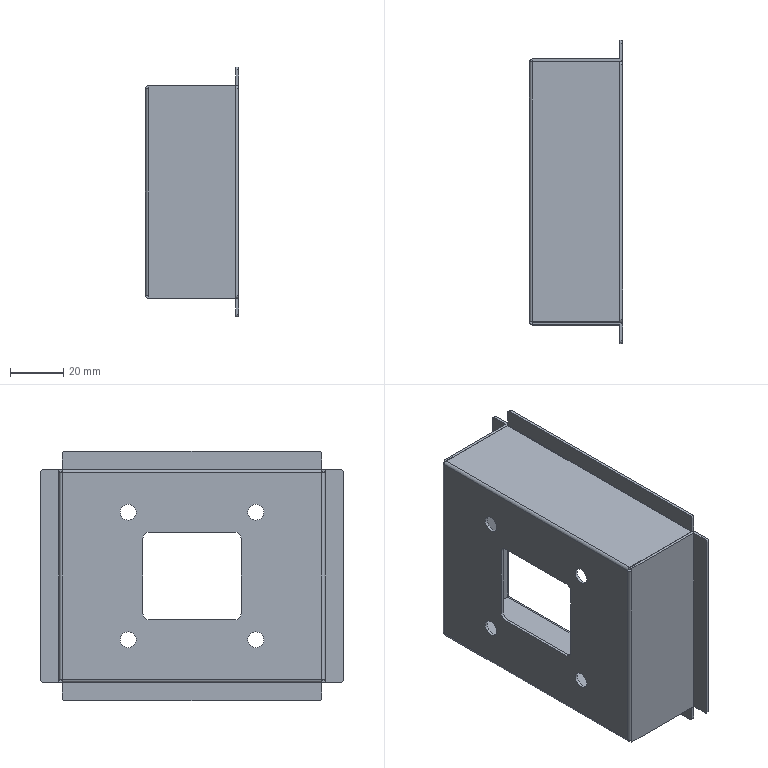Part | STEP file | HESS-408-70-15W-W-30-emergency stop switch box | 1 solid | 78 faces | box 35 x 114 x 94 mm | volume 21062 mm3 | plane 42 | cylinder 36 | commonest cylinder face diameters 0.2 x8 2 x8 2.2 x8 6 x8 5 x4